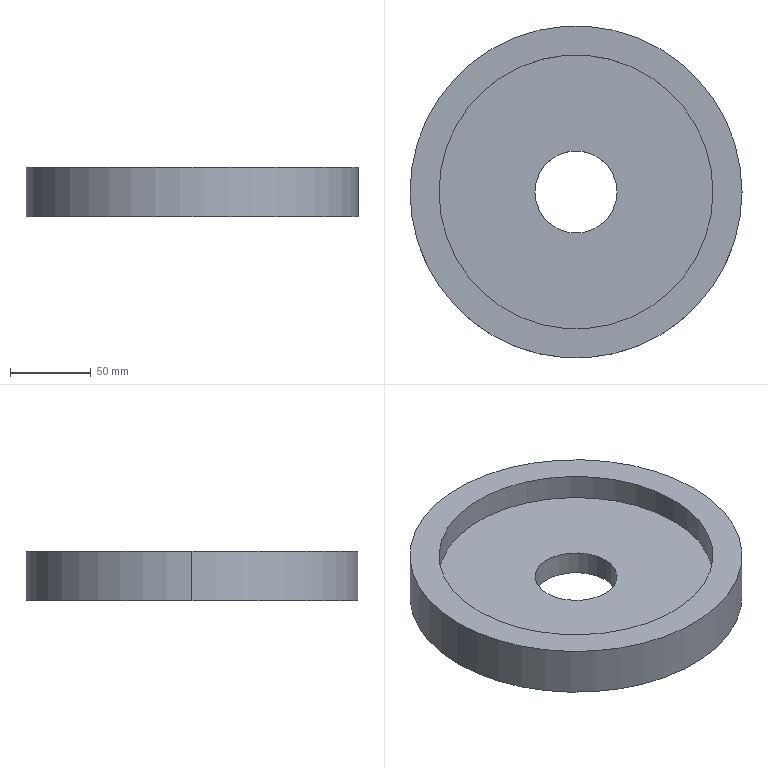Part | SolidWorks | features Extrusion 1, ICE 1 | 1 solid | 9 faces | box 206 x 206 x 31 mm | volume 639393 mm3 | cylinder 6 | plane 3 | commonest cylinder face diameters 51 x2 170 x2 206 x2
STEP:
#1=CARTESIAN_POINT('',(-85.,0.,31.));
#2=VERTEX_POINT('',#1);
#3=CARTESIAN_POINT('',(85.,0.,31.));
#4=VERTEX_POINT('',#3);
#5=CARTESIAN_POINT('',(0.,0.,31.));
#6=DIRECTION('',(0.,0.,1.));
#7=DIRECTION('',(1.,0.,0.));
#8=AXIS2_PLACEMENT_3D('',#5,#6,#7);
#9=CIRCLE('',#8,85.);
#10=EDGE_CURVE('',#2,#4,#9,.T.);
#11=ORIENTED_EDGE('',*,*,#10,.T.);
#12=CARTESIAN_POINT('',(85.,0.,15.));
#13=VERTEX_POINT('',#12);
#14=CARTESIAN_POINT('',(85.,0.,31.));
#15=DIRECTION('',(0.,0.,-1.));
#16=VECTOR('',#15,1000.);
#17=LINE('',#14,#16);
#18=EDGE_CURVE('',#4,#13,#17,.T.);
#19=ORIENTED_EDGE('',*,*,#18,.T.);
#20=CARTESIAN_POINT('',(-85.,0.,15.));
#21=VERTEX_POINT('',#20);
#22=CARTESIAN_POINT('',(0.,0.,15.));
#23=DIRECTION('',(0.,0.,-1.));
#24=DIRECTION('',(1.,0.,0.));
#25=AXIS2_PLACEMENT_3D('',#22,#23,#24);
#26=CIRCLE('',#25,85.);
#27=EDGE_CURVE('',#13,#21,#26,.T.);
#28=ORIENTED_EDGE('',*,*,#27,.T.);
#29=CARTESIAN_POINT('',(-85.,0.,31.));
#30=DIRECTION('',(0.,0.,-1.));
#31=VECTOR('',#30,1000.);
#32=LINE('',#29,#31);
#33=EDGE_CURVE('',#2,#21,#32,.T.);
#34=ORIENTED_EDGE('',*,*,#33,.F.);
#35=EDGE_LOOP('',(#11,#19,#28,#34));
#36=FACE_OUTER_BOUND('',#35,.T.);
#37=CARTESIAN_POINT('',(0.,0.,31.));
#38=DIRECTION('',(0.,0.,-1.));
#39=DIRECTION('',(-1.,0.,0.));
#40=AXIS2_PLACEMENT_3D('',#37,#38,#39);
#41=CYLINDRICAL_SURFACE('',#40,85.);
#42=ADVANCED_FACE('',(#36),#41,.F.);
#43=CARTESIAN_POINT('',(-25.5,0.,15.));
#44=VERTEX_POINT('',#43);
#45=CARTESIAN_POINT('',(25.5,0.,15.));
#46=VERTEX_POINT('',#45);
#47=CARTESIAN_POINT('',(0.,0.,15.));
#48=DIRECTION('',(0.,0.,1.));
#49=DIRECTION('',(1.,0.,0.));
#50=AXIS2_PLACEMENT_3D('',#47,#48,#49);
#51=CIRCLE('',#50,25.5);
#52=EDGE_CURVE('',#44,#46,#51,.T.);
#53=ORIENTED_EDGE('',*,*,#52,.T.);
#54=CARTESIAN_POINT('',(25.5,0.,0.));
#55=VERTEX_POINT('',#54);
#56=CARTESIAN_POINT('',(25.5,0.,15.));
#57=DIRECTION('',(0.,0.,-1.));
#58=VECTOR('',#57,1000.);
#59=LINE('',#56,#58);
#60=EDGE_CURVE('',#46,#55,#59,.T.);
#61=ORIENTED_EDGE('',*,*,#60,.T.);
#62=CARTESIAN_POINT('',(-25.5,0.,0.));
#63=VERTEX_POINT('',#62);
#64=CARTESIAN_POINT('',(0.,0.,0.));
#65=DIRECTION('',(0.,0.,1.));
#66=DIRECTION('',(1.,0.,0.));
#67=AXIS2_PLACEMENT_3D('',#64,#65,#66);
#68=CIRCLE('',#67,25.5);
#69=EDGE_CURVE('',#63,#55,#68,.T.);
#70=ORIENTED_EDGE('',*,*,#69,.F.);
#71=CARTESIAN_POINT('',(-25.5,0.,15.));
#72=DIRECTION('',(0.,0.,-1.));
#73=VECTOR('',#72,1000.);
#74=LINE('',#71,#73);
#75=EDGE_CURVE('',#44,#63,#74,.T.);
#76=ORIENTED_EDGE('',*,*,#75,.F.);
#77=EDGE_LOOP('',(#53,#61,#70,#76));
#78=FACE_OUTER_BOUND('',#77,.T.);
#79=CARTESIAN_POINT('',(0.,0.,15.));
#80=DIRECTION('',(0.,0.,-1.));
#81=DIRECTION('',(-1.,0.,0.));
#82=AXIS2_PLACEMENT_3D('',#79,#80,#81);
#83=CYLINDRICAL_SURFACE('',#82,25.5);
#84=ADVANCED_FACE('',(#78),#83,.F.);
#85=CARTESIAN_POINT('',(103.,0.,31.));
#86=VERTEX_POINT('',#85);
#87=CARTESIAN_POINT('',(-103.,0.,31.));
#88=VERTEX_POINT('',#87);
#89=CARTESIAN_POINT('',(0.,0.,31.));
#90=DIRECTION('',(0.,0.,1.));
#91=DIRECTION('',(1.,0.,0.));
#92=AXIS2_PLACEMENT_3D('',#89,#90,#91);
#93=CIRCLE('',#92,103.);
#94=EDGE_CURVE('',#86,#88,#93,.T.);
#95=ORIENTED_EDGE('',*,*,#94,.F.);
#96=CARTESIAN_POINT('',(103.,0.,0.));
#97=VERTEX_POINT('',#96);
#98=CARTESIAN_POINT('',(103.,0.,15.));
#99=DIRECTION('',(0.,0.,-1.));
#100=VECTOR('',#99,1000.);
#101=LINE('',#98,#100);
#102=EDGE_CURVE('',#86,#97,#101,.T.);
#103=ORIENTED_EDGE('',*,*,#102,.T.);
#104=CARTESIAN_POINT('',(-103.,0.,0.));
#105=VERTEX_POINT('',#104);
#106=CARTESIAN_POINT('',(0.,0.,0.));
#107=DIRECTION('',(0.,0.,1.));
#108=DIRECTION('',(1.,0.,0.));
#109=AXIS2_PLACEMENT_3D('',#106,#107,#108);
#110=CIRCLE('',#109,103.);
#111=EDGE_CURVE('',#97,#105,#110,.T.);
#112=ORIENTED_EDGE('',*,*,#111,.T.);
#113=CARTESIAN_POINT('',(-103.,0.,15.));
#114=DIRECTION('',(0.,0.,-1.));
#115=VECTOR('',#114,1000.);
#116=LINE('',#113,#115);
#117=EDGE_CURVE('',#88,#105,#116,.T.);
#118=ORIENTED_EDGE('',*,*,#117,.F.);
#119=EDGE_LOOP('',(#95,#103,#112,#118));
#120=FACE_OUTER_BOUND('',#119,.T.);
#121=CARTESIAN_POINT('',(0.,0.,15.));
#122=DIRECTION('',(0.,0.,-1.));
#123=DIRECTION('',(-1.,0.,0.));
#124=AXIS2_PLACEMENT_3D('',#121,#122,#123);
#125=CYLINDRICAL_SURFACE('',#124,103.);
#126=ADVANCED_FACE('',(#120),#125,.T.);
#127=ORIENTED_EDGE('',*,*,#52,.F.);
#128=CARTESIAN_POINT('',(0.,0.,15.));
#129=DIRECTION('',(0.,0.,1.));
#130=DIRECTION('',(1.,0.,0.));
#131=AXIS2_PLACEMENT_3D('',#128,#129,#130);
#132=CIRCLE('',#131,25.5);
#133=EDGE_CURVE('',#46,#44,#132,.T.);
#134=ORIENTED_EDGE('',*,*,#133,.F.);
#135=EDGE_LOOP('',(#127,#134));
#136=FACE_BOUND('',#135,.T.);
#137=CARTESIAN_POINT('',(0.,0.,15.));
#138=DIRECTION('',(0.,0.,-1.));
#139=DIRECTION('',(1.,0.,0.));
#140=AXIS2_PLACEMENT_3D('',#137,#138,#139);
#141=CIRCLE('',#140,85.);
#142=EDGE_CURVE('',#21,#13,#141,.T.);
#143=ORIENTED_EDGE('',*,*,#142,.F.);
#144=ORIENTED_EDGE('',*,*,#27,.F.);
#145=EDGE_LOOP('',(#143,#144));
#146=FACE_OUTER_BOUND('',#145,.T.);
#147=CARTESIAN_POINT('',(0.,0.,15.));
#148=DIRECTION('',(0.,0.,1.));
#149=DIRECTION('',(1.,0.,0.));
#150=AXIS2_PLACEMENT_3D('',#147,#148,#149);
#151=PLANE('',#150);
#152=ADVANCED_FACE('',(#136,#146),#151,.T.);
#153=CARTESIAN_POINT('',(0.,0.,0.));
#154=DIRECTION('',(0.,0.,1.));
#155=DIRECTION('',(1.,0.,0.));
#156=AXIS2_PLACEMENT_3D('',#153,#154,#155);
#157=CIRCLE('',#156,103.);
#158=EDGE_CURVE('',#105,#97,#157,.T.);
#159=ORIENTED_EDGE('',*,*,#158,.F.);
#160=ORIENTED_EDGE('',*,*,#111,.F.);
#161=EDGE_LOOP('',(#159,#160));
#162=FACE_OUTER_BOUND('',#161,.T.);
#163=ORIENTED_EDGE('',*,*,#69,.T.);
#164=CARTESIAN_POINT('',(0.,0.,0.));
#165=DIRECTION('',(0.,0.,1.));
#166=DIRECTION('',(1.,0.,0.));
#167=AXIS2_PLACEMENT_3D('',#164,#165,#166);
#168=CIRCLE('',#167,25.5);
#169=EDGE_CURVE('',#55,#63,#168,.T.);
#170=ORIENTED_EDGE('',*,*,#169,.T.);
#171=EDGE_LOOP('',(#163,#170));
#172=FACE_BOUND('',#171,.T.);
#173=CARTESIAN_POINT('',(0.,0.,0.));
#174=DIRECTION('',(0.,0.,1.));
#175=DIRECTION('',(1.,0.,0.));
#176=AXIS2_PLACEMENT_3D('',#173,#174,#175);
#177=PLANE('',#176);
#178=ADVANCED_FACE('',(#162,#172),#177,.F.);
#179=ORIENTED_EDGE('',*,*,#102,.F.);
#180=CARTESIAN_POINT('',(0.,0.,31.));
#181=DIRECTION('',(0.,0.,1.));
#182=DIRECTION('',(1.,0.,0.));
#183=AXIS2_PLACEMENT_3D('',#180,#181,#182);
#184=CIRCLE('',#183,103.);
#185=EDGE_CURVE('',#88,#86,#184,.T.);
#186=ORIENTED_EDGE('',*,*,#185,.F.);
#187=ORIENTED_EDGE('',*,*,#117,.T.);
#188=ORIENTED_EDGE('',*,*,#158,.T.);
#189=EDGE_LOOP('',(#179,#186,#187,#188));
#190=FACE_OUTER_BOUND('',#189,.T.);
#191=CARTESIAN_POINT('',(0.,0.,15.));
#192=DIRECTION('',(0.,0.,-1.));
#193=DIRECTION('',(-1.,0.,0.));
#194=AXIS2_PLACEMENT_3D('',#191,#192,#193);
#195=CYLINDRICAL_SURFACE('',#194,103.);
#196=ADVANCED_FACE('',(#190),#195,.T.);
#197=ORIENTED_EDGE('',*,*,#60,.F.);
#198=ORIENTED_EDGE('',*,*,#133,.T.);
#199=ORIENTED_EDGE('',*,*,#75,.T.);
#200=ORIENTED_EDGE('',*,*,#169,.F.);
#201=EDGE_LOOP('',(#197,#198,#199,#200));
#202=FACE_OUTER_BOUND('',#201,.T.);
#203=CARTESIAN_POINT('',(0.,0.,15.));
#204=DIRECTION('',(0.,0.,-1.));
#205=DIRECTION('',(-1.,0.,0.));
#206=AXIS2_PLACEMENT_3D('',#203,#204,#205);
#207=CYLINDRICAL_SURFACE('',#206,25.5);
#208=ADVANCED_FACE('',(#202),#207,.F.);
#209=ORIENTED_EDGE('',*,*,#185,.T.);
#210=ORIENTED_EDGE('',*,*,#94,.T.);
#211=EDGE_LOOP('',(#209,#210));
#212=FACE_OUTER_BOUND('',#211,.T.);
#213=ORIENTED_EDGE('',*,*,#10,.F.);
#214=CARTESIAN_POINT('',(0.,0.,31.));
#215=DIRECTION('',(0.,0.,1.));
#216=DIRECTION('',(1.,0.,0.));
#217=AXIS2_PLACEMENT_3D('',#214,#215,#216);
#218=CIRCLE('',#217,85.);
#219=EDGE_CURVE('',#4,#2,#218,.T.);
#220=ORIENTED_EDGE('',*,*,#219,.F.);
#221=EDGE_LOOP('',(#213,#220));
#222=FACE_BOUND('',#221,.T.);
#223=CARTESIAN_POINT('',(0.,0.,31.));
#224=DIRECTION('',(0.,0.,1.));
#225=DIRECTION('',(1.,0.,0.));
#226=AXIS2_PLACEMENT_3D('',#223,#224,#225);
#227=PLANE('',#226);
#228=ADVANCED_FACE('',(#212,#222),#227,.T.);
#229=ORIENTED_EDGE('',*,*,#18,.F.);
#230=ORIENTED_EDGE('',*,*,#219,.T.);
#231=ORIENTED_EDGE('',*,*,#33,.T.);
#232=ORIENTED_EDGE('',*,*,#142,.T.);
#233=EDGE_LOOP('',(#229,#230,#231,#232));
#234=FACE_OUTER_BOUND('',#233,.T.);
#235=CARTESIAN_POINT('',(0.,0.,31.));
#236=DIRECTION('',(0.,0.,-1.));
#237=DIRECTION('',(-1.,0.,0.));
#238=AXIS2_PLACEMENT_3D('',#235,#236,#237);
#239=CYLINDRICAL_SURFACE('',#238,85.);
#240=ADVANCED_FACE('',(#234),#239,.F.);
#241=CLOSED_SHELL('',(#42,#84,#126,#152,#178,#196,#208,#228,#240));
#242=MANIFOLD_SOLID_BREP('',#241);
#243=CARTESIAN_POINT('',(0.,0.,0.));
#244=DIRECTION('',(0.,0.,1.));
#245=DIRECTION('',(1.,0.,0.));
#246=AXIS2_PLACEMENT_3D('',#243,#244,#245);
#247=(LENGTH_UNIT()NAMED_UNIT(*)SI_UNIT(.MILLI.,.METRE.));
#248=UNCERTAINTY_MEASURE_WITH_UNIT(LENGTH_MEASURE(0.00001),#247,'','');
#249=(NAMED_UNIT(*)PLANE_ANGLE_UNIT()SI_UNIT($,.RADIAN.));
#250=(NAMED_UNIT(*)SI_UNIT($,.STERADIAN.)SOLID_ANGLE_UNIT());
#251=(GEOMETRIC_REPRESENTATION_CONTEXT(3)GLOBAL_UNCERTAINTY_ASSIGNED_CONTEXT((#248))GLOBAL_UNIT_ASSIGNED_CONTEXT((#247,#249,#250))REPRESENTATION_CONTEXT('',''));
#252=ADVANCED_BREP_SHAPE_REPRESENTATION('',(#242,#246),#251);